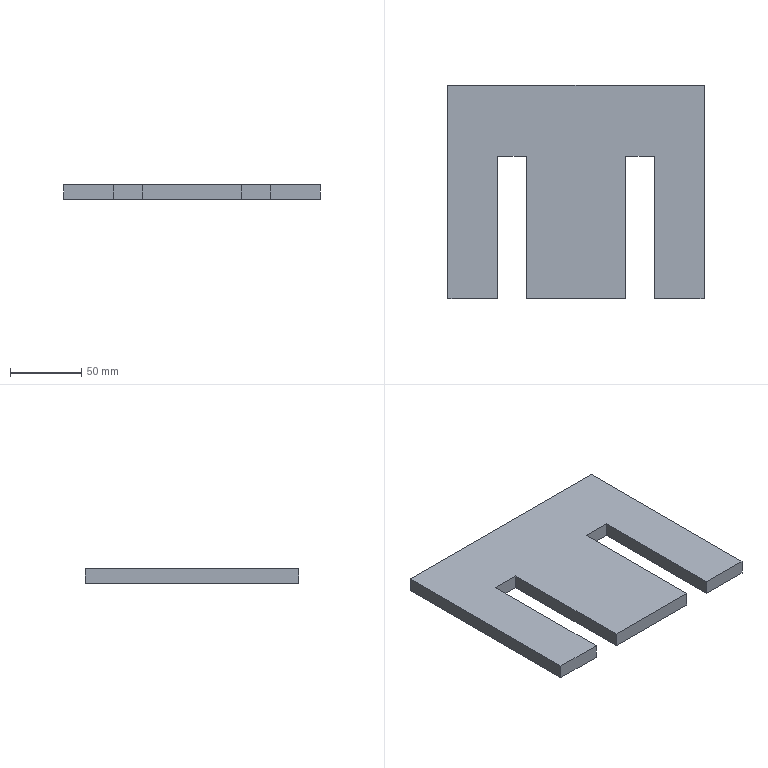Part | SolidWorks | features Extrusion 1, ICE 1, MirrorPattern 1 | 1 solid | 14 faces | box 180 x 150 x 10 mm | volume 230000 mm3 | plane 14
STEP:
#1=CARTESIAN_POINT('',(55.,-75.,0.));
#2=VERTEX_POINT('',#1);
#3=CARTESIAN_POINT('',(55.,-75.,10.));
#4=VERTEX_POINT('',#3);
#5=CARTESIAN_POINT('',(55.,-75.,-0.001));
#6=DIRECTION('',(0.,0.,1.));
#7=VECTOR('',#6,1000.);
#8=LINE('',#5,#7);
#9=EDGE_CURVE('',#2,#4,#8,.T.);
#10=ORIENTED_EDGE('',*,*,#9,.F.);
#11=CARTESIAN_POINT('',(90.,-75.,0.));
#12=VERTEX_POINT('',#11);
#13=CARTESIAN_POINT('',(-90.,-75.,0.));
#14=DIRECTION('',(1.,0.,0.));
#15=VECTOR('',#14,1000.);
#16=LINE('',#13,#15);
#17=EDGE_CURVE('',#2,#12,#16,.T.);
#18=ORIENTED_EDGE('',*,*,#17,.T.);
#19=CARTESIAN_POINT('',(90.,-75.,10.));
#20=VERTEX_POINT('',#19);
#21=CARTESIAN_POINT('',(90.,-75.,10.));
#22=DIRECTION('',(0.,0.,-1.));
#23=VECTOR('',#22,1000.);
#24=LINE('',#21,#23);
#25=EDGE_CURVE('',#20,#12,#24,.T.);
#26=ORIENTED_EDGE('',*,*,#25,.F.);
#27=CARTESIAN_POINT('',(-90.,-75.,10.));
#28=DIRECTION('',(1.,0.,0.));
#29=VECTOR('',#28,1000.);
#30=LINE('',#27,#29);
#31=EDGE_CURVE('',#4,#20,#30,.T.);
#32=ORIENTED_EDGE('',*,*,#31,.F.);
#33=EDGE_LOOP('',(#10,#18,#26,#32));
#34=FACE_OUTER_BOUND('',#33,.T.);
#35=CARTESIAN_POINT('',(-90.,-75.,10.));
#36=DIRECTION('',(0.,1.,0.));
#37=DIRECTION('',(0.,0.,1.));
#38=AXIS2_PLACEMENT_3D('',#35,#36,#37);
#39=PLANE('',#38);
#40=ADVANCED_FACE('',(#34),#39,.F.);
#41=CARTESIAN_POINT('',(35.,-75.,0.));
#42=VERTEX_POINT('',#41);
#43=CARTESIAN_POINT('',(35.,-75.,10.));
#44=VERTEX_POINT('',#43);
#45=CARTESIAN_POINT('',(35.,-75.,-0.001));
#46=DIRECTION('',(0.,0.,1.));
#47=VECTOR('',#46,1000.);
#48=LINE('',#45,#47);
#49=EDGE_CURVE('',#42,#44,#48,.T.);
#50=ORIENTED_EDGE('',*,*,#49,.T.);
#51=CARTESIAN_POINT('',(-35.,-75.,10.));
#52=VERTEX_POINT('',#51);
#53=CARTESIAN_POINT('',(-90.,-75.,10.));
#54=DIRECTION('',(1.,0.,0.));
#55=VECTOR('',#54,1000.);
#56=LINE('',#53,#55);
#57=EDGE_CURVE('',#52,#44,#56,.T.);
#58=ORIENTED_EDGE('',*,*,#57,.F.);
#59=CARTESIAN_POINT('',(-35.,-75.,0.));
#60=VERTEX_POINT('',#59);
#61=CARTESIAN_POINT('',(-35.,-75.,-0.001));
#62=DIRECTION('',(0.,0.,1.));
#63=VECTOR('',#62,1000.);
#64=LINE('',#61,#63);
#65=EDGE_CURVE('',#60,#52,#64,.T.);
#66=ORIENTED_EDGE('',*,*,#65,.F.);
#67=CARTESIAN_POINT('',(-90.,-75.,0.));
#68=DIRECTION('',(1.,0.,0.));
#69=VECTOR('',#68,1000.);
#70=LINE('',#67,#69);
#71=EDGE_CURVE('',#60,#42,#70,.T.);
#72=ORIENTED_EDGE('',*,*,#71,.T.);
#73=EDGE_LOOP('',(#50,#58,#66,#72));
#74=FACE_OUTER_BOUND('',#73,.T.);
#75=CARTESIAN_POINT('',(-90.,-75.,10.));
#76=DIRECTION('',(0.,1.,0.));
#77=DIRECTION('',(0.,0.,1.));
#78=AXIS2_PLACEMENT_3D('',#75,#76,#77);
#79=PLANE('',#78);
#80=ADVANCED_FACE('',(#74),#79,.F.);
#81=CARTESIAN_POINT('',(55.,25.,10.));
#82=VERTEX_POINT('',#81);
#83=CARTESIAN_POINT('',(55.,-75.,10.));
#84=DIRECTION('',(0.,-1.,0.));
#85=VECTOR('',#84,1000.);
#86=LINE('',#83,#85);
#87=EDGE_CURVE('',#82,#4,#86,.T.);
#88=ORIENTED_EDGE('',*,*,#87,.T.);
#89=ORIENTED_EDGE('',*,*,#31,.T.);
#90=CARTESIAN_POINT('',(90.,75.,10.));
#91=VERTEX_POINT('',#90);
#92=CARTESIAN_POINT('',(90.,-75.,10.));
#93=DIRECTION('',(0.,1.,0.));
#94=VECTOR('',#93,1000.);
#95=LINE('',#92,#94);
#96=EDGE_CURVE('',#20,#91,#95,.T.);
#97=ORIENTED_EDGE('',*,*,#96,.T.);
#98=CARTESIAN_POINT('',(-90.,75.,10.));
#99=VERTEX_POINT('',#98);
#100=CARTESIAN_POINT('',(-90.,75.,10.));
#101=DIRECTION('',(-1.,0.,0.));
#102=VECTOR('',#101,1000.);
#103=LINE('',#100,#102);
#104=EDGE_CURVE('',#91,#99,#103,.T.);
#105=ORIENTED_EDGE('',*,*,#104,.T.);
#106=CARTESIAN_POINT('',(-90.,-75.,10.));
#107=VERTEX_POINT('',#106);
#108=CARTESIAN_POINT('',(-90.,-75.,10.));
#109=DIRECTION('',(0.,-1.,0.));
#110=VECTOR('',#109,1000.);
#111=LINE('',#108,#110);
#112=EDGE_CURVE('',#99,#107,#111,.T.);
#113=ORIENTED_EDGE('',*,*,#112,.T.);
#114=CARTESIAN_POINT('',(-55.,-75.,10.));
#115=VERTEX_POINT('',#114);
#116=CARTESIAN_POINT('',(-90.,-75.,10.));
#117=DIRECTION('',(1.,0.,0.));
#118=VECTOR('',#117,1000.);
#119=LINE('',#116,#118);
#120=EDGE_CURVE('',#107,#115,#119,.T.);
#121=ORIENTED_EDGE('',*,*,#120,.T.);
#122=CARTESIAN_POINT('',(-55.,25.,10.));
#123=VERTEX_POINT('',#122);
#124=CARTESIAN_POINT('',(-55.,-75.,10.));
#125=DIRECTION('',(0.,-1.,0.));
#126=VECTOR('',#125,1000.);
#127=LINE('',#124,#126);
#128=EDGE_CURVE('',#123,#115,#127,.T.);
#129=ORIENTED_EDGE('',*,*,#128,.F.);
#130=CARTESIAN_POINT('',(-35.,25.,10.));
#131=VERTEX_POINT('',#130);
#132=CARTESIAN_POINT('',(-55.,25.,10.));
#133=DIRECTION('',(-1.,0.,0.));
#134=VECTOR('',#133,1000.);
#135=LINE('',#132,#134);
#136=EDGE_CURVE('',#131,#123,#135,.T.);
#137=ORIENTED_EDGE('',*,*,#136,.F.);
#138=CARTESIAN_POINT('',(-35.,-75.,10.));
#139=DIRECTION('',(0.,1.,0.));
#140=VECTOR('',#139,1000.);
#141=LINE('',#138,#140);
#142=EDGE_CURVE('',#52,#131,#141,.T.);
#143=ORIENTED_EDGE('',*,*,#142,.F.);
#144=ORIENTED_EDGE('',*,*,#57,.T.);
#145=CARTESIAN_POINT('',(35.,25.,10.));
#146=VERTEX_POINT('',#145);
#147=CARTESIAN_POINT('',(35.,-75.,10.));
#148=DIRECTION('',(0.,1.,0.));
#149=VECTOR('',#148,1000.);
#150=LINE('',#147,#149);
#151=EDGE_CURVE('',#44,#146,#150,.T.);
#152=ORIENTED_EDGE('',*,*,#151,.T.);
#153=CARTESIAN_POINT('',(55.,25.,10.));
#154=DIRECTION('',(1.,0.,0.));
#155=VECTOR('',#154,1000.);
#156=LINE('',#153,#155);
#157=EDGE_CURVE('',#146,#82,#156,.T.);
#158=ORIENTED_EDGE('',*,*,#157,.T.);
#159=EDGE_LOOP('',(#88,#89,#97,#105,#113,#121,#129,#137,#143,#144,#152,#158));
#160=FACE_OUTER_BOUND('',#159,.T.);
#161=CARTESIAN_POINT('',(0.,0.,10.));
#162=DIRECTION('',(0.,0.,-1.));
#163=DIRECTION('',(-1.,0.,0.));
#164=AXIS2_PLACEMENT_3D('',#161,#162,#163);
#165=PLANE('',#164);
#166=ADVANCED_FACE('',(#160),#165,.F.);
#167=ORIENTED_EDGE('',*,*,#17,.F.);
#168=CARTESIAN_POINT('',(55.,25.,0.));
#169=VERTEX_POINT('',#168);
#170=CARTESIAN_POINT('',(55.,-75.,0.));
#171=DIRECTION('',(0.,-1.,0.));
#172=VECTOR('',#171,1000.);
#173=LINE('',#170,#172);
#174=EDGE_CURVE('',#169,#2,#173,.T.);
#175=ORIENTED_EDGE('',*,*,#174,.F.);
#176=CARTESIAN_POINT('',(35.,25.,0.));
#177=VERTEX_POINT('',#176);
#178=CARTESIAN_POINT('',(55.,25.,0.));
#179=DIRECTION('',(1.,0.,0.));
#180=VECTOR('',#179,1000.);
#181=LINE('',#178,#180);
#182=EDGE_CURVE('',#177,#169,#181,.T.);
#183=ORIENTED_EDGE('',*,*,#182,.F.);
#184=CARTESIAN_POINT('',(35.,-75.,0.));
#185=DIRECTION('',(0.,1.,0.));
#186=VECTOR('',#185,1000.);
#187=LINE('',#184,#186);
#188=EDGE_CURVE('',#42,#177,#187,.T.);
#189=ORIENTED_EDGE('',*,*,#188,.F.);
#190=ORIENTED_EDGE('',*,*,#71,.F.);
#191=CARTESIAN_POINT('',(-35.,25.,0.));
#192=VERTEX_POINT('',#191);
#193=CARTESIAN_POINT('',(-35.,-75.,0.));
#194=DIRECTION('',(0.,1.,0.));
#195=VECTOR('',#194,1000.);
#196=LINE('',#193,#195);
#197=EDGE_CURVE('',#60,#192,#196,.T.);
#198=ORIENTED_EDGE('',*,*,#197,.T.);
#199=CARTESIAN_POINT('',(-55.,25.,0.));
#200=VERTEX_POINT('',#199);
#201=CARTESIAN_POINT('',(-55.,25.,0.));
#202=DIRECTION('',(-1.,0.,0.));
#203=VECTOR('',#202,1000.);
#204=LINE('',#201,#203);
#205=EDGE_CURVE('',#192,#200,#204,.T.);
#206=ORIENTED_EDGE('',*,*,#205,.T.);
#207=CARTESIAN_POINT('',(-55.,-75.,0.));
#208=VERTEX_POINT('',#207);
#209=CARTESIAN_POINT('',(-55.,-75.,0.));
#210=DIRECTION('',(0.,-1.,0.));
#211=VECTOR('',#210,1000.);
#212=LINE('',#209,#211);
#213=EDGE_CURVE('',#200,#208,#212,.T.);
#214=ORIENTED_EDGE('',*,*,#213,.T.);
#215=CARTESIAN_POINT('',(-90.,-75.,0.));
#216=VERTEX_POINT('',#215);
#217=CARTESIAN_POINT('',(-90.,-75.,0.));
#218=DIRECTION('',(1.,0.,0.));
#219=VECTOR('',#218,1000.);
#220=LINE('',#217,#219);
#221=EDGE_CURVE('',#216,#208,#220,.T.);
#222=ORIENTED_EDGE('',*,*,#221,.F.);
#223=CARTESIAN_POINT('',(-90.,75.,0.));
#224=VERTEX_POINT('',#223);
#225=CARTESIAN_POINT('',(-90.,-75.,0.));
#226=DIRECTION('',(0.,-1.,0.));
#227=VECTOR('',#226,1000.);
#228=LINE('',#225,#227);
#229=EDGE_CURVE('',#224,#216,#228,.T.);
#230=ORIENTED_EDGE('',*,*,#229,.F.);
#231=CARTESIAN_POINT('',(90.,75.,0.));
#232=VERTEX_POINT('',#231);
#233=CARTESIAN_POINT('',(-90.,75.,0.));
#234=DIRECTION('',(-1.,0.,0.));
#235=VECTOR('',#234,1000.);
#236=LINE('',#233,#235);
#237=EDGE_CURVE('',#232,#224,#236,.T.);
#238=ORIENTED_EDGE('',*,*,#237,.F.);
#239=CARTESIAN_POINT('',(90.,-75.,0.));
#240=DIRECTION('',(0.,1.,0.));
#241=VECTOR('',#240,1000.);
#242=LINE('',#239,#241);
#243=EDGE_CURVE('',#12,#232,#242,.T.);
#244=ORIENTED_EDGE('',*,*,#243,.F.);
#245=EDGE_LOOP('',(#167,#175,#183,#189,#190,#198,#206,#214,#222,#230,#238,#244));
#246=FACE_OUTER_BOUND('',#245,.T.);
#247=CARTESIAN_POINT('',(0.,0.,0.));
#248=DIRECTION('',(0.,0.,-1.));
#249=DIRECTION('',(-1.,0.,0.));
#250=AXIS2_PLACEMENT_3D('',#247,#248,#249);
#251=PLANE('',#250);
#252=ADVANCED_FACE('',(#246),#251,.T.);
#253=ORIENTED_EDGE('',*,*,#221,.T.);
#254=CARTESIAN_POINT('',(-55.,-75.,-0.001));
#255=DIRECTION('',(0.,0.,1.));
#256=VECTOR('',#255,1000.);
#257=LINE('',#254,#256);
#258=EDGE_CURVE('',#208,#115,#257,.T.);
#259=ORIENTED_EDGE('',*,*,#258,.T.);
#260=ORIENTED_EDGE('',*,*,#120,.F.);
#261=CARTESIAN_POINT('',(-90.,-75.,10.));
#262=DIRECTION('',(0.,0.,-1.));
#263=VECTOR('',#262,1000.);
#264=LINE('',#261,#263);
#265=EDGE_CURVE('',#107,#216,#264,.T.);
#266=ORIENTED_EDGE('',*,*,#265,.T.);
#267=EDGE_LOOP('',(#253,#259,#260,#266));
#268=FACE_OUTER_BOUND('',#267,.T.);
#269=CARTESIAN_POINT('',(-90.,-75.,10.));
#270=DIRECTION('',(0.,1.,0.));
#271=DIRECTION('',(0.,0.,1.));
#272=AXIS2_PLACEMENT_3D('',#269,#270,#271);
#273=PLANE('',#272);
#274=ADVANCED_FACE('',(#268),#273,.F.);
#275=ORIENTED_EDGE('',*,*,#243,.T.);
#276=CARTESIAN_POINT('',(90.,75.,10.));
#277=DIRECTION('',(0.,0.,-1.));
#278=VECTOR('',#277,1000.);
#279=LINE('',#276,#278);
#280=EDGE_CURVE('',#91,#232,#279,.T.);
#281=ORIENTED_EDGE('',*,*,#280,.F.);
#282=ORIENTED_EDGE('',*,*,#96,.F.);
#283=ORIENTED_EDGE('',*,*,#25,.T.);
#284=EDGE_LOOP('',(#275,#281,#282,#283));
#285=FACE_OUTER_BOUND('',#284,.T.);
#286=CARTESIAN_POINT('',(90.,-75.,10.));
#287=DIRECTION('',(-1.,0.,0.));
#288=DIRECTION('',(0.,0.,1.));
#289=AXIS2_PLACEMENT_3D('',#286,#287,#288);
#290=PLANE('',#289);
#291=ADVANCED_FACE('',(#285),#290,.F.);
#292=ORIENTED_EDGE('',*,*,#237,.T.);
#293=CARTESIAN_POINT('',(-90.,75.,10.));
#294=DIRECTION('',(0.,0.,-1.));
#295=VECTOR('',#294,1000.);
#296=LINE('',#293,#295);
#297=EDGE_CURVE('',#99,#224,#296,.T.);
#298=ORIENTED_EDGE('',*,*,#297,.F.);
#299=ORIENTED_EDGE('',*,*,#104,.F.);
#300=ORIENTED_EDGE('',*,*,#280,.T.);
#301=EDGE_LOOP('',(#292,#298,#299,#300));
#302=FACE_OUTER_BOUND('',#301,.T.);
#303=CARTESIAN_POINT('',(-90.,75.,10.));
#304=DIRECTION('',(0.,-1.,0.));
#305=DIRECTION('',(0.,0.,-1.));
#306=AXIS2_PLACEMENT_3D('',#303,#304,#305);
#307=PLANE('',#306);
#308=ADVANCED_FACE('',(#302),#307,.F.);
#309=ORIENTED_EDGE('',*,*,#229,.T.);
#310=ORIENTED_EDGE('',*,*,#265,.F.);
#311=ORIENTED_EDGE('',*,*,#112,.F.);
#312=ORIENTED_EDGE('',*,*,#297,.T.);
#313=EDGE_LOOP('',(#309,#310,#311,#312));
#314=FACE_OUTER_BOUND('',#313,.T.);
#315=CARTESIAN_POINT('',(-90.,-75.,10.));
#316=DIRECTION('',(1.,0.,0.));
#317=DIRECTION('',(0.,0.,-1.));
#318=AXIS2_PLACEMENT_3D('',#315,#316,#317);
#319=PLANE('',#318);
#320=ADVANCED_FACE('',(#314),#319,.F.);
#321=CARTESIAN_POINT('',(-55.,25.,-0.001));
#322=DIRECTION('',(0.,0.,1.));
#323=VECTOR('',#322,1000.);
#324=LINE('',#321,#323);
#325=EDGE_CURVE('',#200,#123,#324,.T.);
#326=ORIENTED_EDGE('',*,*,#325,.T.);
#327=ORIENTED_EDGE('',*,*,#128,.T.);
#328=ORIENTED_EDGE('',*,*,#258,.F.);
#329=ORIENTED_EDGE('',*,*,#213,.F.);
#330=EDGE_LOOP('',(#326,#327,#328,#329));
#331=FACE_OUTER_BOUND('',#330,.T.);
#332=CARTESIAN_POINT('',(-55.,-75.,-0.001));
#333=DIRECTION('',(-1.,0.,0.));
#334=DIRECTION('',(0.,0.,1.));
#335=AXIS2_PLACEMENT_3D('',#332,#333,#334);
#336=PLANE('',#335);
#337=ADVANCED_FACE('',(#331),#336,.F.);
#338=CARTESIAN_POINT('',(-35.,25.,-0.001));
#339=DIRECTION('',(0.,0.,1.));
#340=VECTOR('',#339,1000.);
#341=LINE('',#338,#340);
#342=EDGE_CURVE('',#192,#131,#341,.T.);
#343=ORIENTED_EDGE('',*,*,#342,.T.);
#344=ORIENTED_EDGE('',*,*,#136,.T.);
#345=ORIENTED_EDGE('',*,*,#325,.F.);
#346=ORIENTED_EDGE('',*,*,#205,.F.);
#347=EDGE_LOOP('',(#343,#344,#345,#346));
#348=FACE_OUTER_BOUND('',#347,.T.);
#349=CARTESIAN_POINT('',(-55.,25.,-0.001));
#350=DIRECTION('',(0.,1.,0.));
#351=DIRECTION('',(0.,0.,1.));
#352=AXIS2_PLACEMENT_3D('',#349,#350,#351);
#353=PLANE('',#352);
#354=ADVANCED_FACE('',(#348),#353,.F.);
#355=ORIENTED_EDGE('',*,*,#65,.T.);
#356=ORIENTED_EDGE('',*,*,#142,.T.);
#357=ORIENTED_EDGE('',*,*,#342,.F.);
#358=ORIENTED_EDGE('',*,*,#197,.F.);
#359=EDGE_LOOP('',(#355,#356,#357,#358));
#360=FACE_OUTER_BOUND('',#359,.T.);
#361=CARTESIAN_POINT('',(-35.,-75.,-0.001));
#362=DIRECTION('',(1.,0.,0.));
#363=DIRECTION('',(0.,0.,-1.));
#364=AXIS2_PLACEMENT_3D('',#361,#362,#363);
#365=PLANE('',#364);
#366=ADVANCED_FACE('',(#360),#365,.F.);
#367=ORIENTED_EDGE('',*,*,#174,.T.);
#368=ORIENTED_EDGE('',*,*,#9,.T.);
#369=ORIENTED_EDGE('',*,*,#87,.F.);
#370=CARTESIAN_POINT('',(55.,25.,-0.001));
#371=DIRECTION('',(0.,0.,1.));
#372=VECTOR('',#371,1000.);
#373=LINE('',#370,#372);
#374=EDGE_CURVE('',#169,#82,#373,.T.);
#375=ORIENTED_EDGE('',*,*,#374,.F.);
#376=EDGE_LOOP('',(#367,#368,#369,#375));
#377=FACE_OUTER_BOUND('',#376,.T.);
#378=CARTESIAN_POINT('',(55.,-75.,-0.001));
#379=DIRECTION('',(-1.,0.,0.));
#380=DIRECTION('',(0.,0.,1.));
#381=AXIS2_PLACEMENT_3D('',#378,#379,#380);
#382=PLANE('',#381);
#383=ADVANCED_FACE('',(#377),#382,.T.);
#384=ORIENTED_EDGE('',*,*,#188,.T.);
#385=CARTESIAN_POINT('',(35.,25.,-0.001));
#386=DIRECTION('',(0.,0.,1.));
#387=VECTOR('',#386,1000.);
#388=LINE('',#385,#387);
#389=EDGE_CURVE('',#177,#146,#388,.T.);
#390=ORIENTED_EDGE('',*,*,#389,.T.);
#391=ORIENTED_EDGE('',*,*,#151,.F.);
#392=ORIENTED_EDGE('',*,*,#49,.F.);
#393=EDGE_LOOP('',(#384,#390,#391,#392));
#394=FACE_OUTER_BOUND('',#393,.T.);
#395=CARTESIAN_POINT('',(35.,-75.,-0.001));
#396=DIRECTION('',(1.,0.,0.));
#397=DIRECTION('',(0.,0.,-1.));
#398=AXIS2_PLACEMENT_3D('',#395,#396,#397);
#399=PLANE('',#398);
#400=ADVANCED_FACE('',(#394),#399,.T.);
#401=ORIENTED_EDGE('',*,*,#182,.T.);
#402=ORIENTED_EDGE('',*,*,#374,.T.);
#403=ORIENTED_EDGE('',*,*,#157,.F.);
#404=ORIENTED_EDGE('',*,*,#389,.F.);
#405=EDGE_LOOP('',(#401,#402,#403,#404));
#406=FACE_OUTER_BOUND('',#405,.T.);
#407=CARTESIAN_POINT('',(55.,25.,-0.001));
#408=DIRECTION('',(0.,-1.,0.));
#409=DIRECTION('',(0.,0.,-1.));
#410=AXIS2_PLACEMENT_3D('',#407,#408,#409);
#411=PLANE('',#410);
#412=ADVANCED_FACE('',(#406),#411,.T.);
#413=CLOSED_SHELL('',(#40,#80,#166,#252,#274,#291,#308,#320,#337,#354,#366,#383,#400,#412));
#414=MANIFOLD_SOLID_BREP('',#413);
#415=CARTESIAN_POINT('',(0.,0.,0.));
#416=DIRECTION('',(0.,0.,1.));
#417=DIRECTION('',(1.,0.,0.));
#418=AXIS2_PLACEMENT_3D('',#415,#416,#417);
#419=(LENGTH_UNIT()NAMED_UNIT(*)SI_UNIT(.MILLI.,.METRE.));
#420=UNCERTAINTY_MEASURE_WITH_UNIT(LENGTH_MEASURE(0.00001),#419,'','');
#421=(NAMED_UNIT(*)PLANE_ANGLE_UNIT()SI_UNIT($,.RADIAN.));
#422=(NAMED_UNIT(*)SI_UNIT($,.STERADIAN.)SOLID_ANGLE_UNIT());
#423=(GEOMETRIC_REPRESENTATION_CONTEXT(3)GLOBAL_UNCERTAINTY_ASSIGNED_CONTEXT((#420))GLOBAL_UNIT_ASSIGNED_CONTEXT((#419,#421,#422))REPRESENTATION_CONTEXT('',''));
#424=ADVANCED_BREP_SHAPE_REPRESENTATION('',(#414,#418),#423);